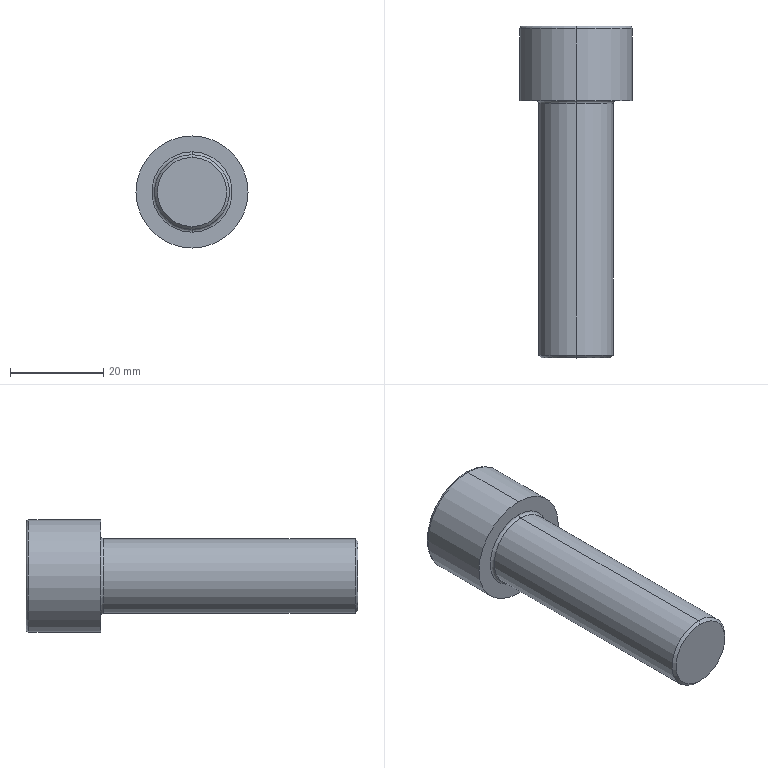Part | STEP file | 1 solid | 20 faces | box 24 x 71 x 24 mm | volume 16928 mm3 | plane 10 | torus 4 | cylinder 4 | cone 2 | commonest cylinder face diameters 16 x2 24 x2
STEP:
#1=CARTESIAN_POINT('',(0.,-55.,-7.4));
#2=VERTEX_POINT('',#1);
#3=CARTESIAN_POINT('',(0.,-55.,7.4));
#4=VERTEX_POINT('',#3);
#5=CARTESIAN_POINT('',(0.,-55.,0.));
#6=DIRECTION('',(0.,-1.,0.));
#7=DIRECTION('',(0.,0.,-1.));
#8=AXIS2_PLACEMENT_3D('',#5,#6,#7);
#9=CIRCLE('',#8,7.4);
#10=EDGE_CURVE('',#2,#4,#9,.T.);
#11=ORIENTED_EDGE('',*,*,#10,.F.);
#12=CARTESIAN_POINT('',(0.,-54.4,-8.));
#13=VERTEX_POINT('',#12);
#14=CARTESIAN_POINT('',(0.,-55.,-7.4));
#15=DIRECTION('',(0.,0.7071,-0.7071));
#16=VECTOR('',#15,1000.);
#17=LINE('',#14,#16);
#18=EDGE_CURVE('',#2,#13,#17,.T.);
#19=ORIENTED_EDGE('',*,*,#18,.T.);
#20=CARTESIAN_POINT('',(0.,-54.4,8.));
#21=VERTEX_POINT('',#20);
#22=CARTESIAN_POINT('',(0.,-54.4,0.));
#23=DIRECTION('',(0.,1.,0.));
#24=DIRECTION('',(0.,0.,-1.));
#25=AXIS2_PLACEMENT_3D('',#22,#23,#24);
#26=CIRCLE('',#25,8.);
#27=EDGE_CURVE('',#21,#13,#26,.T.);
#28=ORIENTED_EDGE('',*,*,#27,.F.);
#29=CARTESIAN_POINT('',(0.,-55.,7.4));
#30=DIRECTION('',(0.,0.7071,0.7071));
#31=VECTOR('',#30,1000.);
#32=LINE('',#29,#31);
#33=EDGE_CURVE('',#4,#21,#32,.T.);
#34=ORIENTED_EDGE('',*,*,#33,.F.);
#35=EDGE_LOOP('',(#11,#19,#28,#34));
#36=FACE_OUTER_BOUND('',#35,.T.);
#37=CARTESIAN_POINT('',(0.,-55.,0.));
#38=DIRECTION('',(0.,1.,0.));
#39=DIRECTION('',(0.,0.,1.));
#40=AXIS2_PLACEMENT_3D('',#37,#38,#39);
#41=CONICAL_SURFACE('',#40,7.4,0.7854);
#42=ADVANCED_FACE('',(#36),#41,.T.);
#43=CARTESIAN_POINT('',(0.,15.4,-12.));
#44=VERTEX_POINT('',#43);
#45=CARTESIAN_POINT('',(0.,15.4,12.));
#46=VERTEX_POINT('',#45);
#47=CARTESIAN_POINT('',(0.,15.4,0.));
#48=DIRECTION('',(0.,-1.,0.));
#49=DIRECTION('',(0.,0.,1.));
#50=AXIS2_PLACEMENT_3D('',#47,#48,#49);
#51=CIRCLE('',#50,12.);
#52=EDGE_CURVE('',#44,#46,#51,.T.);
#53=ORIENTED_EDGE('',*,*,#52,.F.);
#54=CARTESIAN_POINT('',(0.,16.,-11.4));
#55=VERTEX_POINT('',#54);
#56=CARTESIAN_POINT('',(0.,15.4,-11.4));
#57=DIRECTION('',(1.,0.,0.));
#58=DIRECTION('',(0.,0.,-1.));
#59=AXIS2_PLACEMENT_3D('',#56,#57,#58);
#60=CIRCLE('',#59,0.6);
#61=EDGE_CURVE('',#44,#55,#60,.T.);
#62=ORIENTED_EDGE('',*,*,#61,.T.);
#63=CARTESIAN_POINT('',(0.,16.,11.4));
#64=VERTEX_POINT('',#63);
#65=CARTESIAN_POINT('',(0.,16.,0.));
#66=DIRECTION('',(0.,1.,0.));
#67=DIRECTION('',(0.,0.,1.));
#68=AXIS2_PLACEMENT_3D('',#65,#66,#67);
#69=CIRCLE('',#68,11.4);
#70=EDGE_CURVE('',#64,#55,#69,.T.);
#71=ORIENTED_EDGE('',*,*,#70,.F.);
#72=CARTESIAN_POINT('',(0.,15.4,11.4));
#73=DIRECTION('',(-1.,0.,0.));
#74=DIRECTION('',(0.,0.,1.));
#75=AXIS2_PLACEMENT_3D('',#72,#73,#74);
#76=CIRCLE('',#75,0.6);
#77=EDGE_CURVE('',#46,#64,#76,.T.);
#78=ORIENTED_EDGE('',*,*,#77,.F.);
#79=EDGE_LOOP('',(#53,#62,#71,#78));
#80=FACE_OUTER_BOUND('',#79,.T.);
#81=CARTESIAN_POINT('',(0.,15.4,0.));
#82=DIRECTION('',(0.,1.,0.));
#83=DIRECTION('',(0.,0.,1.));
#84=AXIS2_PLACEMENT_3D('',#81,#82,#83);
#85=TOROIDAL_SURFACE('',#84,11.4,0.6);
#86=ADVANCED_FACE('',(#80),#85,.T.);
#87=CARTESIAN_POINT('',(0.,-0.6,8.));
#88=VERTEX_POINT('',#87);
#89=CARTESIAN_POINT('',(0.,-0.6,-8.));
#90=VERTEX_POINT('',#89);
#91=CARTESIAN_POINT('',(0.,-0.6,0.));
#92=DIRECTION('',(0.,-1.,0.));
#93=DIRECTION('',(0.,0.,-1.));
#94=AXIS2_PLACEMENT_3D('',#91,#92,#93);
#95=CIRCLE('',#94,8.);
#96=EDGE_CURVE('',#88,#90,#95,.T.);
#97=ORIENTED_EDGE('',*,*,#96,.F.);
#98=CARTESIAN_POINT('',(0.,0.,8.6));
#99=VERTEX_POINT('',#98);
#100=CARTESIAN_POINT('',(0.,-0.6,8.6));
#101=DIRECTION('',(1.,0.,0.));
#102=DIRECTION('',(0.,0.,-1.));
#103=AXIS2_PLACEMENT_3D('',#100,#101,#102);
#104=CIRCLE('',#103,0.6);
#105=EDGE_CURVE('',#88,#99,#104,.T.);
#106=ORIENTED_EDGE('',*,*,#105,.T.);
#107=CARTESIAN_POINT('',(0.,0.,-8.6));
#108=VERTEX_POINT('',#107);
#109=CARTESIAN_POINT('',(0.,0.,0.));
#110=DIRECTION('',(0.,1.,0.));
#111=DIRECTION('',(0.,0.,-1.));
#112=AXIS2_PLACEMENT_3D('',#109,#110,#111);
#113=CIRCLE('',#112,8.6);
#114=EDGE_CURVE('',#108,#99,#113,.T.);
#115=ORIENTED_EDGE('',*,*,#114,.F.);
#116=CARTESIAN_POINT('',(0.,-0.6,-8.6));
#117=DIRECTION('',(-1.,0.,0.));
#118=DIRECTION('',(0.,0.,1.));
#119=AXIS2_PLACEMENT_3D('',#116,#117,#118);
#120=CIRCLE('',#119,0.6);
#121=EDGE_CURVE('',#90,#108,#120,.T.);
#122=ORIENTED_EDGE('',*,*,#121,.F.);
#123=EDGE_LOOP('',(#97,#106,#115,#122));
#124=FACE_OUTER_BOUND('',#123,.T.);
#125=CARTESIAN_POINT('',(0.,-0.6,0.));
#126=DIRECTION('',(0.,-1.,0.));
#127=DIRECTION('',(0.,0.,-1.));
#128=AXIS2_PLACEMENT_3D('',#125,#126,#127);
#129=TOROIDAL_SURFACE('',#128,8.6,0.6);
#130=ADVANCED_FACE('',(#124),#129,.F.);
#131=CARTESIAN_POINT('',(0.,-0.6,0.));
#132=DIRECTION('',(0.,-1.,0.));
#133=DIRECTION('',(0.,0.,-1.));
#134=AXIS2_PLACEMENT_3D('',#131,#132,#133);
#135=CIRCLE('',#134,8.);
#136=EDGE_CURVE('',#90,#88,#135,.T.);
#137=ORIENTED_EDGE('',*,*,#136,.T.);
#138=CARTESIAN_POINT('',(0.,0.,8.));
#139=DIRECTION('',(0.,-1.,0.));
#140=VECTOR('',#139,1000.);
#141=LINE('',#138,#140);
#142=EDGE_CURVE('',#88,#21,#141,.T.);
#143=ORIENTED_EDGE('',*,*,#142,.T.);
#144=ORIENTED_EDGE('',*,*,#27,.T.);
#145=CARTESIAN_POINT('',(0.,0.,-8.));
#146=DIRECTION('',(0.,-1.,0.));
#147=VECTOR('',#146,1000.);
#148=LINE('',#145,#147);
#149=EDGE_CURVE('',#90,#13,#148,.T.);
#150=ORIENTED_EDGE('',*,*,#149,.F.);
#151=EDGE_LOOP('',(#137,#143,#144,#150));
#152=FACE_OUTER_BOUND('',#151,.T.);
#153=CARTESIAN_POINT('',(0.,0.,0.));
#154=DIRECTION('',(0.,-1.,0.));
#155=DIRECTION('',(0.,0.,-1.));
#156=AXIS2_PLACEMENT_3D('',#153,#154,#155);
#157=CYLINDRICAL_SURFACE('',#156,8.);
#158=ADVANCED_FACE('',(#152),#157,.T.);
#159=ORIENTED_EDGE('',*,*,#52,.T.);
#160=CARTESIAN_POINT('',(0.,0.,12.));
#161=VERTEX_POINT('',#160);
#162=CARTESIAN_POINT('',(0.,0.,12.));
#163=DIRECTION('',(0.,-1.,0.));
#164=VECTOR('',#163,1000.);
#165=LINE('',#162,#164);
#166=EDGE_CURVE('',#46,#161,#165,.T.);
#167=ORIENTED_EDGE('',*,*,#166,.T.);
#168=CARTESIAN_POINT('',(0.,0.,-12.));
#169=VERTEX_POINT('',#168);
#170=CARTESIAN_POINT('',(0.,0.,0.));
#171=DIRECTION('',(0.,-1.,0.));
#172=DIRECTION('',(0.,0.,-1.));
#173=AXIS2_PLACEMENT_3D('',#170,#171,#172);
#174=CIRCLE('',#173,12.);
#175=EDGE_CURVE('',#169,#161,#174,.T.);
#176=ORIENTED_EDGE('',*,*,#175,.F.);
#177=CARTESIAN_POINT('',(0.,0.,-12.));
#178=DIRECTION('',(0.,-1.,0.));
#179=VECTOR('',#178,1000.);
#180=LINE('',#177,#179);
#181=EDGE_CURVE('',#44,#169,#180,.T.);
#182=ORIENTED_EDGE('',*,*,#181,.F.);
#183=EDGE_LOOP('',(#159,#167,#176,#182));
#184=FACE_OUTER_BOUND('',#183,.T.);
#185=CARTESIAN_POINT('',(0.,0.,0.));
#186=DIRECTION('',(0.,-1.,0.));
#187=DIRECTION('',(0.,0.,-1.));
#188=AXIS2_PLACEMENT_3D('',#185,#186,#187);
#189=CYLINDRICAL_SURFACE('',#188,12.);
#190=ADVANCED_FACE('',(#184),#189,.T.);
#191=ORIENTED_EDGE('',*,*,#70,.T.);
#192=CARTESIAN_POINT('',(0.,16.,0.));
#193=DIRECTION('',(0.,1.,0.));
#194=DIRECTION('',(0.,0.,1.));
#195=AXIS2_PLACEMENT_3D('',#192,#193,#194);
#196=CIRCLE('',#195,11.4);
#197=EDGE_CURVE('',#55,#64,#196,.T.);
#198=ORIENTED_EDGE('',*,*,#197,.T.);
#199=EDGE_LOOP('',(#191,#198));
#200=FACE_OUTER_BOUND('',#199,.T.);
#201=CARTESIAN_POINT('',(0.,16.,-8.083));
#202=VERTEX_POINT('',#201);
#203=CARTESIAN_POINT('',(-7.,16.,-4.041));
#204=VERTEX_POINT('',#203);
#205=CARTESIAN_POINT('',(0.,16.,-8.083));
#206=DIRECTION('',(-0.866,0.,0.5));
#207=VECTOR('',#206,1000.);
#208=LINE('',#205,#207);
#209=EDGE_CURVE('',#202,#204,#208,.T.);
#210=ORIENTED_EDGE('',*,*,#209,.F.);
#211=CARTESIAN_POINT('',(7.,16.,-4.041));
#212=VERTEX_POINT('',#211);
#213=CARTESIAN_POINT('',(7.,16.,-4.041));
#214=DIRECTION('',(-0.866,0.,-0.5));
#215=VECTOR('',#214,1000.);
#216=LINE('',#213,#215);
#217=EDGE_CURVE('',#212,#202,#216,.T.);
#218=ORIENTED_EDGE('',*,*,#217,.F.);
#219=CARTESIAN_POINT('',(7.,16.,4.041));
#220=VERTEX_POINT('',#219);
#221=CARTESIAN_POINT('',(7.,16.,4.041));
#222=DIRECTION('',(0.,0.,-1.));
#223=VECTOR('',#222,1000.);
#224=LINE('',#221,#223);
#225=EDGE_CURVE('',#220,#212,#224,.T.);
#226=ORIENTED_EDGE('',*,*,#225,.F.);
#227=CARTESIAN_POINT('',(0.,16.,8.083));
#228=VERTEX_POINT('',#227);
#229=CARTESIAN_POINT('',(0.,16.,8.083));
#230=DIRECTION('',(0.866,0.,-0.5));
#231=VECTOR('',#230,1000.);
#232=LINE('',#229,#231);
#233=EDGE_CURVE('',#228,#220,#232,.T.);
#234=ORIENTED_EDGE('',*,*,#233,.F.);
#235=CARTESIAN_POINT('',(-7.,16.,4.041));
#236=VERTEX_POINT('',#235);
#237=CARTESIAN_POINT('',(-7.,16.,4.041));
#238=DIRECTION('',(0.866,0.,0.5));
#239=VECTOR('',#238,1000.);
#240=LINE('',#237,#239);
#241=EDGE_CURVE('',#236,#228,#240,.T.);
#242=ORIENTED_EDGE('',*,*,#241,.F.);
#243=CARTESIAN_POINT('',(-7.,16.,-4.041));
#244=DIRECTION('',(0.,0.,1.));
#245=VECTOR('',#244,1000.);
#246=LINE('',#243,#245);
#247=EDGE_CURVE('',#204,#236,#246,.T.);
#248=ORIENTED_EDGE('',*,*,#247,.F.);
#249=EDGE_LOOP('',(#210,#218,#226,#234,#242,#248));
#250=FACE_BOUND('',#249,.T.);
#251=CARTESIAN_POINT('',(0.,16.,0.));
#252=DIRECTION('',(0.,1.,0.));
#253=DIRECTION('',(0.,0.,1.));
#254=AXIS2_PLACEMENT_3D('',#251,#252,#253);
#255=PLANE('',#254);
#256=ADVANCED_FACE('',(#200,#250),#255,.T.);
#257=ORIENTED_EDGE('',*,*,#166,.F.);
#258=CARTESIAN_POINT('',(0.,15.4,0.));
#259=DIRECTION('',(0.,-1.,0.));
#260=DIRECTION('',(0.,0.,1.));
#261=AXIS2_PLACEMENT_3D('',#258,#259,#260);
#262=CIRCLE('',#261,12.);
#263=EDGE_CURVE('',#46,#44,#262,.T.);
#264=ORIENTED_EDGE('',*,*,#263,.T.);
#265=ORIENTED_EDGE('',*,*,#181,.T.);
#266=CARTESIAN_POINT('',(0.,0.,0.));
#267=DIRECTION('',(0.,-1.,0.));
#268=DIRECTION('',(0.,0.,-1.));
#269=AXIS2_PLACEMENT_3D('',#266,#267,#268);
#270=CIRCLE('',#269,12.);
#271=EDGE_CURVE('',#161,#169,#270,.T.);
#272=ORIENTED_EDGE('',*,*,#271,.F.);
#273=EDGE_LOOP('',(#257,#264,#265,#272));
#274=FACE_OUTER_BOUND('',#273,.T.);
#275=CARTESIAN_POINT('',(0.,0.,0.));
#276=DIRECTION('',(0.,-1.,0.));
#277=DIRECTION('',(0.,0.,-1.));
#278=AXIS2_PLACEMENT_3D('',#275,#276,#277);
#279=CYLINDRICAL_SURFACE('',#278,12.);
#280=ADVANCED_FACE('',(#274),#279,.T.);
#281=ORIENTED_EDGE('',*,*,#114,.T.);
#282=CARTESIAN_POINT('',(0.,0.,0.));
#283=DIRECTION('',(0.,1.,0.));
#284=DIRECTION('',(0.,0.,-1.));
#285=AXIS2_PLACEMENT_3D('',#282,#283,#284);
#286=CIRCLE('',#285,8.6);
#287=EDGE_CURVE('',#99,#108,#286,.T.);
#288=ORIENTED_EDGE('',*,*,#287,.T.);
#289=EDGE_LOOP('',(#281,#288));
#290=FACE_BOUND('',#289,.T.);
#291=ORIENTED_EDGE('',*,*,#175,.T.);
#292=ORIENTED_EDGE('',*,*,#271,.T.);
#293=EDGE_LOOP('',(#291,#292));
#294=FACE_OUTER_BOUND('',#293,.T.);
#295=CARTESIAN_POINT('',(12.,0.,0.));
#296=DIRECTION('',(0.,-1.,0.));
#297=DIRECTION('',(0.,0.,-1.));
#298=AXIS2_PLACEMENT_3D('',#295,#296,#297);
#299=PLANE('',#298);
#300=ADVANCED_FACE('',(#290,#294),#299,.T.);
#301=ORIENTED_EDGE('',*,*,#142,.F.);
#302=ORIENTED_EDGE('',*,*,#96,.T.);
#303=ORIENTED_EDGE('',*,*,#149,.T.);
#304=CARTESIAN_POINT('',(0.,-54.4,0.));
#305=DIRECTION('',(0.,1.,0.));
#306=DIRECTION('',(0.,0.,-1.));
#307=AXIS2_PLACEMENT_3D('',#304,#305,#306);
#308=CIRCLE('',#307,8.);
#309=EDGE_CURVE('',#13,#21,#308,.T.);
#310=ORIENTED_EDGE('',*,*,#309,.T.);
#311=EDGE_LOOP('',(#301,#302,#303,#310));
#312=FACE_OUTER_BOUND('',#311,.T.);
#313=CARTESIAN_POINT('',(0.,0.,0.));
#314=DIRECTION('',(0.,-1.,0.));
#315=DIRECTION('',(0.,0.,-1.));
#316=AXIS2_PLACEMENT_3D('',#313,#314,#315);
#317=CYLINDRICAL_SURFACE('',#316,8.);
#318=ADVANCED_FACE('',(#312),#317,.T.);
#319=CARTESIAN_POINT('',(0.,-55.,0.));
#320=DIRECTION('',(0.,-1.,0.));
#321=DIRECTION('',(0.,0.,-1.));
#322=AXIS2_PLACEMENT_3D('',#319,#320,#321);
#323=CIRCLE('',#322,7.4);
#324=EDGE_CURVE('',#4,#2,#323,.T.);
#325=ORIENTED_EDGE('',*,*,#324,.T.);
#326=ORIENTED_EDGE('',*,*,#10,.T.);
#327=EDGE_LOOP('',(#325,#326));
#328=FACE_OUTER_BOUND('',#327,.T.);
#329=CARTESIAN_POINT('',(8.,-55.,0.));
#330=DIRECTION('',(0.,-1.,0.));
#331=DIRECTION('',(0.,0.,-1.));
#332=AXIS2_PLACEMENT_3D('',#329,#330,#331);
#333=PLANE('',#332);
#334=ADVANCED_FACE('',(#328),#333,.T.);
#335=ORIENTED_EDGE('',*,*,#209,.T.);
#336=CARTESIAN_POINT('',(-7.,8.,-4.041));
#337=VERTEX_POINT('',#336);
#338=CARTESIAN_POINT('',(-7.,8.,-4.041));
#339=DIRECTION('',(0.,1.,0.));
#340=VECTOR('',#339,1000.);
#341=LINE('',#338,#340);
#342=EDGE_CURVE('',#337,#204,#341,.T.);
#343=ORIENTED_EDGE('',*,*,#342,.F.);
#344=CARTESIAN_POINT('',(0.,8.,-8.083));
#345=VERTEX_POINT('',#344);
#346=CARTESIAN_POINT('',(0.,8.,-8.083));
#347=DIRECTION('',(-0.866,0.,0.5));
#348=VECTOR('',#347,1000.);
#349=LINE('',#346,#348);
#350=EDGE_CURVE('',#345,#337,#349,.T.);
#351=ORIENTED_EDGE('',*,*,#350,.F.);
#352=CARTESIAN_POINT('',(0.,8.,-8.083));
#353=DIRECTION('',(0.,1.,0.));
#354=VECTOR('',#353,1000.);
#355=LINE('',#352,#354);
#356=EDGE_CURVE('',#345,#202,#355,.T.);
#357=ORIENTED_EDGE('',*,*,#356,.T.);
#358=EDGE_LOOP('',(#335,#343,#351,#357));
#359=FACE_OUTER_BOUND('',#358,.T.);
#360=CARTESIAN_POINT('',(0.,8.,-8.083));
#361=DIRECTION('',(-0.5,0.,-0.866));
#362=DIRECTION('',(-0.866,0.,0.5));
#363=AXIS2_PLACEMENT_3D('',#360,#361,#362);
#364=PLANE('',#363);
#365=ADVANCED_FACE('',(#359),#364,.F.);
#366=ORIENTED_EDGE('',*,*,#217,.T.);
#367=ORIENTED_EDGE('',*,*,#356,.F.);
#368=CARTESIAN_POINT('',(7.,8.,-4.041));
#369=VERTEX_POINT('',#368);
#370=CARTESIAN_POINT('',(7.,8.,-4.041));
#371=DIRECTION('',(-0.866,0.,-0.5));
#372=VECTOR('',#371,1000.);
#373=LINE('',#370,#372);
#374=EDGE_CURVE('',#369,#345,#373,.T.);
#375=ORIENTED_EDGE('',*,*,#374,.F.);
#376=CARTESIAN_POINT('',(7.,8.,-4.041));
#377=DIRECTION('',(0.,1.,0.));
#378=VECTOR('',#377,1000.);
#379=LINE('',#376,#378);
#380=EDGE_CURVE('',#369,#212,#379,.T.);
#381=ORIENTED_EDGE('',*,*,#380,.T.);
#382=EDGE_LOOP('',(#366,#367,#375,#381));
#383=FACE_OUTER_BOUND('',#382,.T.);
#384=CARTESIAN_POINT('',(7.,8.,-4.041));
#385=DIRECTION('',(0.5,0.,-0.866));
#386=DIRECTION('',(-0.866,0.,-0.5));
#387=AXIS2_PLACEMENT_3D('',#384,#385,#386);
#388=PLANE('',#387);
#389=ADVANCED_FACE('',(#383),#388,.F.);
#390=ORIENTED_EDGE('',*,*,#225,.T.);
#391=ORIENTED_EDGE('',*,*,#380,.F.);
#392=CARTESIAN_POINT('',(7.,8.,4.041));
#393=VERTEX_POINT('',#392);
#394=CARTESIAN_POINT('',(7.,8.,4.041));
#395=DIRECTION('',(0.,0.,-1.));
#396=VECTOR('',#395,1000.);
#397=LINE('',#394,#396);
#398=EDGE_CURVE('',#393,#369,#397,.T.);
#399=ORIENTED_EDGE('',*,*,#398,.F.);
#400=CARTESIAN_POINT('',(7.,8.,4.041));
#401=DIRECTION('',(0.,1.,0.));
#402=VECTOR('',#401,1000.);
#403=LINE('',#400,#402);
#404=EDGE_CURVE('',#393,#220,#403,.T.);
#405=ORIENTED_EDGE('',*,*,#404,.T.);
#406=EDGE_LOOP('',(#390,#391,#399,#405));
#407=FACE_OUTER_BOUND('',#406,.T.);
#408=CARTESIAN_POINT('',(7.,8.,4.041));
#409=DIRECTION('',(1.,0.,0.));
#410=DIRECTION('',(0.,0.,-1.));
#411=AXIS2_PLACEMENT_3D('',#408,#409,#410);
#412=PLANE('',#411);
#413=ADVANCED_FACE('',(#407),#412,.F.);
#414=ORIENTED_EDGE('',*,*,#233,.T.);
#415=ORIENTED_EDGE('',*,*,#404,.F.);
#416=CARTESIAN_POINT('',(0.,8.,8.083));
#417=VERTEX_POINT('',#416);
#418=CARTESIAN_POINT('',(0.,8.,8.083));
#419=DIRECTION('',(0.866,0.,-0.5));
#420=VECTOR('',#419,1000.);
#421=LINE('',#418,#420);
#422=EDGE_CURVE('',#417,#393,#421,.T.);
#423=ORIENTED_EDGE('',*,*,#422,.F.);
#424=CARTESIAN_POINT('',(0.,8.,8.083));
#425=DIRECTION('',(0.,1.,0.));
#426=VECTOR('',#425,1000.);
#427=LINE('',#424,#426);
#428=EDGE_CURVE('',#417,#228,#427,.T.);
#429=ORIENTED_EDGE('',*,*,#428,.T.);
#430=EDGE_LOOP('',(#414,#415,#423,#429));
#431=FACE_OUTER_BOUND('',#430,.T.);
#432=CARTESIAN_POINT('',(0.,8.,8.083));
#433=DIRECTION('',(0.5,0.,0.866));
#434=DIRECTION('',(0.866,0.,-0.5));
#435=AXIS2_PLACEMENT_3D('',#432,#433,#434);
#436=PLANE('',#435);
#437=ADVANCED_FACE('',(#431),#436,.F.);
#438=ORIENTED_EDGE('',*,*,#241,.T.);
#439=ORIENTED_EDGE('',*,*,#428,.F.);
#440=CARTESIAN_POINT('',(-7.,8.,4.041));
#441=VERTEX_POINT('',#440);
#442=CARTESIAN_POINT('',(-7.,8.,4.041));
#443=DIRECTION('',(0.866,0.,0.5));
#444=VECTOR('',#443,1000.);
#445=LINE('',#442,#444);
#446=EDGE_CURVE('',#441,#417,#445,.T.);
#447=ORIENTED_EDGE('',*,*,#446,.F.);
#448=CARTESIAN_POINT('',(-7.,8.,4.041));
#449=DIRECTION('',(0.,1.,0.));
#450=VECTOR('',#449,1000.);
#451=LINE('',#448,#450);
#452=EDGE_CURVE('',#441,#236,#451,.T.);
#453=ORIENTED_EDGE('',*,*,#452,.T.);
#454=EDGE_LOOP('',(#438,#439,#447,#453));
#455=FACE_OUTER_BOUND('',#454,.T.);
#456=CARTESIAN_POINT('',(-7.,8.,4.041));
#457=DIRECTION('',(-0.5,0.,0.866));
#458=DIRECTION('',(0.866,0.,0.5));
#459=AXIS2_PLACEMENT_3D('',#456,#457,#458);
#460=PLANE('',#459);
#461=ADVANCED_FACE('',(#455),#460,.F.);
#462=ORIENTED_EDGE('',*,*,#247,.T.);
#463=ORIENTED_EDGE('',*,*,#452,.F.);
#464=CARTESIAN_POINT('',(-7.,8.,-4.041));
#465=DIRECTION('',(0.,0.,1.));
#466=VECTOR('',#465,1000.);
#467=LINE('',#464,#466);
#468=EDGE_CURVE('',#337,#441,#467,.T.);
#469=ORIENTED_EDGE('',*,*,#468,.F.);
#470=ORIENTED_EDGE('',*,*,#342,.T.);
#471=EDGE_LOOP('',(#462,#463,#469,#470));
#472=FACE_OUTER_BOUND('',#471,.T.);
#473=CARTESIAN_POINT('',(-7.,8.,-4.041));
#474=DIRECTION('',(-1.,0.,0.));
#475=DIRECTION('',(0.,0.,1.));
#476=AXIS2_PLACEMENT_3D('',#473,#474,#475);
#477=PLANE('',#476);
#478=ADVANCED_FACE('',(#472),#477,.F.);
#479=ORIENTED_EDGE('',*,*,#350,.T.);
#480=ORIENTED_EDGE('',*,*,#468,.T.);
#481=ORIENTED_EDGE('',*,*,#446,.T.);
#482=ORIENTED_EDGE('',*,*,#422,.T.);
#483=ORIENTED_EDGE('',*,*,#398,.T.);
#484=ORIENTED_EDGE('',*,*,#374,.T.);
#485=EDGE_LOOP('',(#479,#480,#481,#482,#483,#484));
#486=FACE_OUTER_BOUND('',#485,.T.);
#487=CARTESIAN_POINT('',(0.,8.,0.));
#488=DIRECTION('',(0.,1.,0.));
#489=DIRECTION('',(0.,0.,1.));
#490=AXIS2_PLACEMENT_3D('',#487,#488,#489);
#491=PLANE('',#490);
#492=ADVANCED_FACE('',(#486),#491,.T.);
#493=ORIENTED_EDGE('',*,*,#105,.F.);
#494=ORIENTED_EDGE('',*,*,#136,.F.);
#495=ORIENTED_EDGE('',*,*,#121,.T.);
#496=ORIENTED_EDGE('',*,*,#287,.F.);
#497=EDGE_LOOP('',(#493,#494,#495,#496));
#498=FACE_OUTER_BOUND('',#497,.T.);
#499=CARTESIAN_POINT('',(0.,-0.6,0.));
#500=DIRECTION('',(0.,-1.,0.));
#501=DIRECTION('',(0.,0.,-1.));
#502=AXIS2_PLACEMENT_3D('',#499,#500,#501);
#503=TOROIDAL_SURFACE('',#502,8.6,0.6);
#504=ADVANCED_FACE('',(#498),#503,.F.);
#505=ORIENTED_EDGE('',*,*,#61,.F.);
#506=ORIENTED_EDGE('',*,*,#263,.F.);
#507=ORIENTED_EDGE('',*,*,#77,.T.);
#508=ORIENTED_EDGE('',*,*,#197,.F.);
#509=EDGE_LOOP('',(#505,#506,#507,#508));
#510=FACE_OUTER_BOUND('',#509,.T.);
#511=CARTESIAN_POINT('',(0.,15.4,0.));
#512=DIRECTION('',(0.,1.,0.));
#513=DIRECTION('',(0.,0.,1.));
#514=AXIS2_PLACEMENT_3D('',#511,#512,#513);
#515=TOROIDAL_SURFACE('',#514,11.4,0.6);
#516=ADVANCED_FACE('',(#510),#515,.T.);
#517=ORIENTED_EDGE('',*,*,#18,.F.);
#518=ORIENTED_EDGE('',*,*,#324,.F.);
#519=ORIENTED_EDGE('',*,*,#33,.T.);
#520=ORIENTED_EDGE('',*,*,#309,.F.);
#521=EDGE_LOOP('',(#517,#518,#519,#520));
#522=FACE_OUTER_BOUND('',#521,.T.);
#523=CARTESIAN_POINT('',(0.,-55.,0.));
#524=DIRECTION('',(0.,1.,0.));
#525=DIRECTION('',(0.,0.,1.));
#526=AXIS2_PLACEMENT_3D('',#523,#524,#525);
#527=CONICAL_SURFACE('',#526,7.4,0.7854);
#528=ADVANCED_FACE('',(#522),#527,.T.);
#529=CLOSED_SHELL('',(#42,#86,#130,#158,#190,#256,#280,#300,#318,#334,#365,#389,#413,#437,#461,#478,#492,#504,#516,#528));
#530=MANIFOLD_SOLID_BREP('',#529);
#531=CARTESIAN_POINT('',(0.,0.,0.));
#532=DIRECTION('',(0.,0.,1.));
#533=DIRECTION('',(1.,0.,0.));
#534=AXIS2_PLACEMENT_3D('',#531,#532,#533);
#535=(LENGTH_UNIT()NAMED_UNIT(*)SI_UNIT(.MILLI.,.METRE.));
#536=UNCERTAINTY_MEASURE_WITH_UNIT(LENGTH_MEASURE(0.00001),#535,'','');
#537=(NAMED_UNIT(*)PLANE_ANGLE_UNIT()SI_UNIT($,.RADIAN.));
#538=(NAMED_UNIT(*)SI_UNIT($,.STERADIAN.)SOLID_ANGLE_UNIT());
#539=(GEOMETRIC_REPRESENTATION_CONTEXT(3)GLOBAL_UNCERTAINTY_ASSIGNED_CONTEXT((#536))GLOBAL_UNIT_ASSIGNED_CONTEXT((#535,#537,#538))REPRESENTATION_CONTEXT('',''));
#540=ADVANCED_BREP_SHAPE_REPRESENTATION('',(#530,#534),#539);